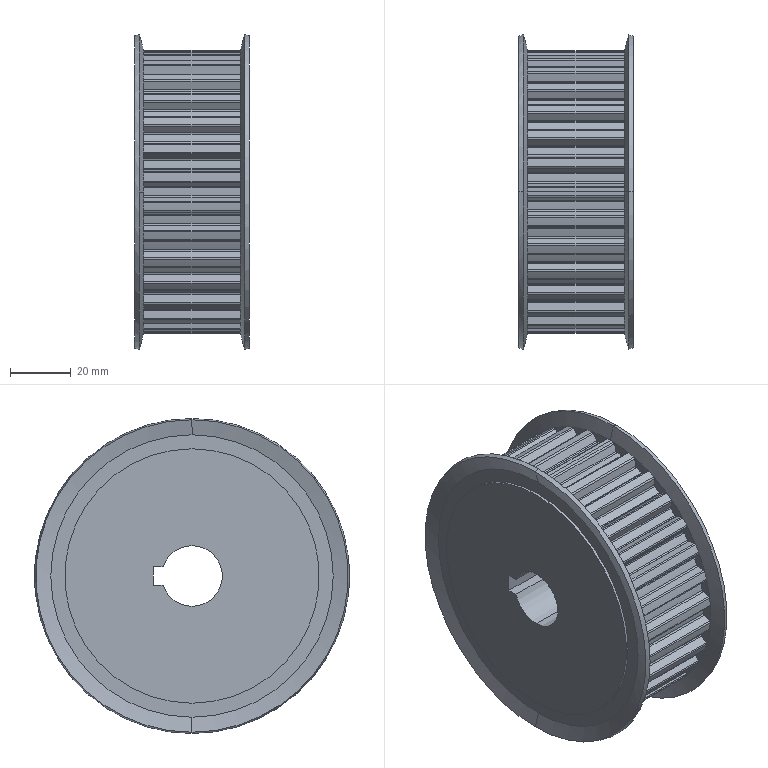Part | SolidWorks | features ICE 2, BaseBody 1 | 1 solid | 347 faces | box 37.864 x 104 x 104 mm | volume 230318 mm3 | cylinder 208 | plane 127 | cone 12 | commonest cylinder face diameters 1 x70 1.2 x70 93.65 x31 87.25 x30 84 x4 20 x3